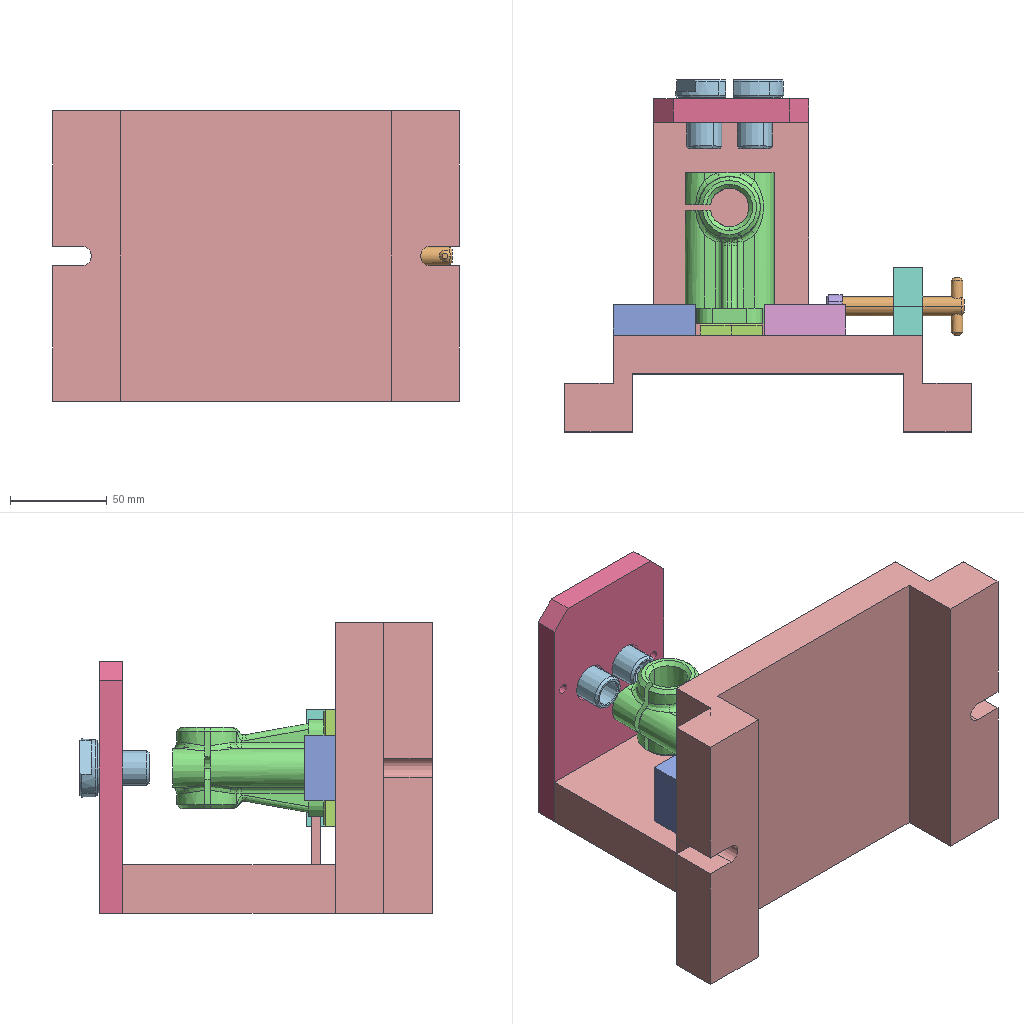Assembly | SolidWorks | 10 different items | 12 placed | box 210 x 182 x 150 mm
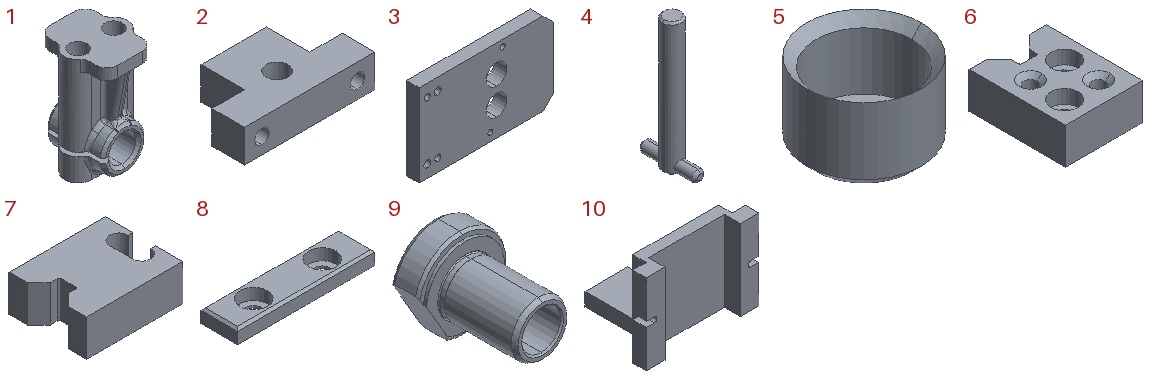Parts list (item | quantity | size | volume | features):
1 | x1 | 46 x 50 x 78 mm | 61833 mm3 | features Fillet 15, ICE 6, Rib 2, Chamfer 1, Extrusion 1
2 | x1 | 60 x 35 x 15 mm | 19468 mm3 | features 3DProfileFeature 1, Extrusion 1, HoleWzd 1, ICE 1
3 | x1 | 130 x 12 x 80 mm | 113262 mm3 | features HoleWzd 3, 3DProfileFeature 2, Chamfer 1, Extrusion 1, ICE 1
4 | x1 | 10 x 30 x 70 mm | 5997 mm3 | features Chamfer 2, Extrusion 1, ICE 1
5 | x1 | 12 x 12 x 8 mm | 320.442 mm3 | features Chamfer 1, Extrusion 1, ICE 1
6 | x1 | 34 x 42.517 x 16 mm | 18300 mm3 | features Chamfer 2, Cut 2, Fillet 2, HoleWzd 2, Extrusion 1, ICE 1
7 | x1 | 42 x 34 x 16 mm | 18899 mm3 | features Cut 2, Fillet 2, Extrusion 1, ICE 1
8 | x2 | 60 x 16 x 6 mm | 4486 mm3 | features Cut 2, Chamfer 1, Extrusion 1, LPattern 1
9 | x2 | 29.63 x 35.75 x 30 mm | 7686 mm3 | features Chamfer 7, Cut 2, Fillet 1, Revolution 1
10 | x1 | 210 x 160 x 150 mm | 964186 mm3 | features HoleWzd 3, ICE 3, Extrusion 1
Mates (type | each side: item.copy, entity, surface, feature):
Coincident | 10.1 face plane Boss-Extrude1 | 6.1 face plane Base-Extrude | 2 times
Parallel | 10.1 face plane Boss-Extrude1 | 6.1 face plane Base-Extrude
DistanceDim | 6.1 face plane Base-Extrude | 10.1 face plane Boss-Extrude1
Coincident | 10.1 face plane Boss-Extrude1 | 8.1 face plane Base-Extrude
Coincident | 10.1 face plane Boss-Extrude1 | 8.2 face plane Base-Extrude
Coincident | 8.1 face plane Base-Extrude | 8.2 face plane Base-Extrude | 2 times
Coincident | 10.1 face plane Boss-Extrude1 | 2.1 face plane Boss-Extrude1 | 2 times
DistanceDim | 2.1 face plane Boss-Extrude1 | 10.1 face plane Boss-Extrude1
Concentric | 4.1 face cylinder Boss-Extrude1 | 5.1 face cylinder Cut-Extrude1
Coincident | 4.1 face plane Boss-Extrude1 | 5.1 face plane Cut-Extrude1
Concentric | 2.1 face cylinder Cut-Extrude1 | 4.1 face cylinder Boss-Extrude1
Coincident | 7.1 face plane Cut-Extrude3 | 5.1 face plane Boss-Extrude1
Parallel | 2.1 face plane Boss-Extrude1 | 4.1 face plane Boss-Extrude2
Concentric | 6.1 face cylinder CBORE for M5 Hex Head Screw2 | assembly face
Coincident | 6.1 face plane CBORE for M5 Hex Head Screw2 | assembly face
Concentric | 6.1 face cylinder CBORE for M5 Hex Head Screw1 | assembly face
Coincident | 6.1 face plane CBORE for M5 Hex Head Screw1 | assembly face
Concentric | 2.1 face cylinder CBORE for M6 Hexagon socket head cap screws1 | assembly face | 2 times
Coincident | 2.1 face plane CBORE for M6 Hexagon socket head cap screws1 | assembly face | 2 times
Concentric | 8.1 face cylinder Cut-Extrude2 | assembly face
Coincident | 8.1 face plane Cut-Extrude2 | assembly face
Concentric | 8.2 face cylinder LPattern1 | assembly face
Coincident | 8.2 face plane LPattern1 | assembly face
Concentric | 8.2 face cylinder Cut-Extrude2 | assembly face
Coincident | 8.2 face plane Cut-Extrude2 | assembly face
Concentric | 8.1 face cylinder LPattern1 | assembly face
Coincident | 8.1 face plane LPattern1 | assembly face
Concentric | 6.1 face cylinder Cut-Extrude4 | assembly face | 2 times
Coincident | 6.1 face plane Base-Extrude | assembly edge
Coincident | 6.1 face plane Base-Extrude | assembly face
Coincident | 8.2 face plane Base-Extrude | 1.1 face plane Boss-Extrude1
Width | 10.1 face plane Boss-Extrude1 | 10.1 face plane Boss-Extrude1 | 1.1 face plane Boss-Extrude1 | 1.1 face plane Boss-Extrude1
Tangent | 7.1 face plane Cut-Extrude1 | 1.1 face cylinder Boss-Extrude2 | 2 times
Tangent | 6.1 face plane Cut-Extrude1 | 1.1 face cylinder Boss-Extrude2
Width | 8.2 face plane Base-Extrude | 8.1 face plane Base-Extrude | 1.1 face plane Boss-Extrude1 | 1.1 face plane Boss-Extrude1
Coincident | 10.1 face plane Boss-Extrude1 | 7.1 face plane Base-Extrude
Coincident | 10.1 face plane Boss-Extrude2 | 3.1 face plane Boss-Extrude1
Coincident | 10.1 face plane Boss-Extrude1 | 3.1 face plane Boss-Extrude1
Width | 10.1 face plane Boss-Extrude2 | 10.1 face plane Boss-Extrude2 | 3.1 face plane Boss-Extrude1 | 3.1 face plane Boss-Extrude1
Concentric | 3.1 face cylinder Ø20.0mm dowel hole 1 | 9.1 face cylinder Base-Revolve
Concentric | 3.1 face cylinder Ø20.0mm dowel hole 1 | 9.2 face cylinder Base-Revolve
Coincident | 3.1 face plane Boss-Extrude1 | 9.2 face plane Base-Revolve
Coincident | 3.1 face plane Boss-Extrude1 | 9.1 face plane Base-Revolve
Parallel | 3.1 face plane Boss-Extrude1 | 9.1 face plane Cut-Extrude2
Parallel | 9.1 face plane Cut-Extrude2 | 9.2 face plane Cut-Extrude2
Concentric | 9.1 face cylinder Base-Revolve | assembly face
Concentric | 9.2 face cylinder Base-Revolve | assembly face
Coincident | 3.1 face plane Boss-Extrude1 | assembly face | 4 times
Coincident | 9.2 face plane Cut-Extrude1 | assembly face
Parallel | 9.2 face plane Cut-Extrude1 | assembly face
Concentric | 3.1 face cylinder Cut-Extrude1 | assembly face | 2 times
Coincident | 9.1 face plane Cut-Extrude1 | assembly face
Parallel | 9.1 face plane Cut-Extrude1 | assembly face
Concentric | 3.1 face cylinder CBORE for M6 Hexagon socket head cap screws1 | assembly face | 2 times
Coincident | 3.1 face plane CBORE for M6 Hexagon socket head cap screws1 | assembly face | 2 times
Concentric | 3.1 face cylinder Ø6.0mm dowel hole 1 | assembly face | 2 times